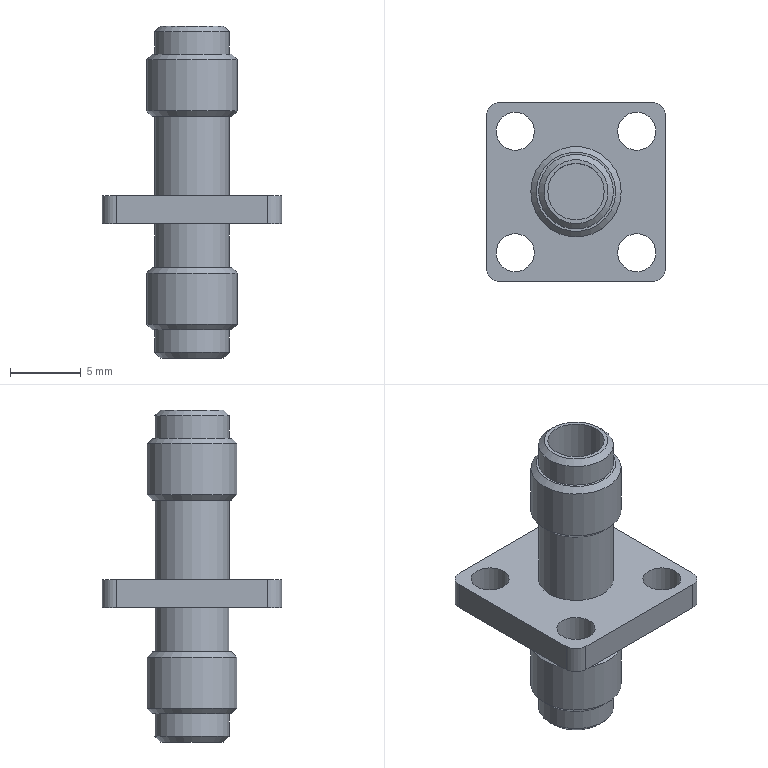Part | STEP file | Connector SMA-KKF | 1 solid | 36 faces | box 12.7 x 12.7 x 23.5 mm | volume 626.237 mm3 | cylinder 16 | plane 14 | cone 6 | commonest cylinder face diameters 2 x4 2.7 x4 5.3 x4 4 x2 6.4 x2